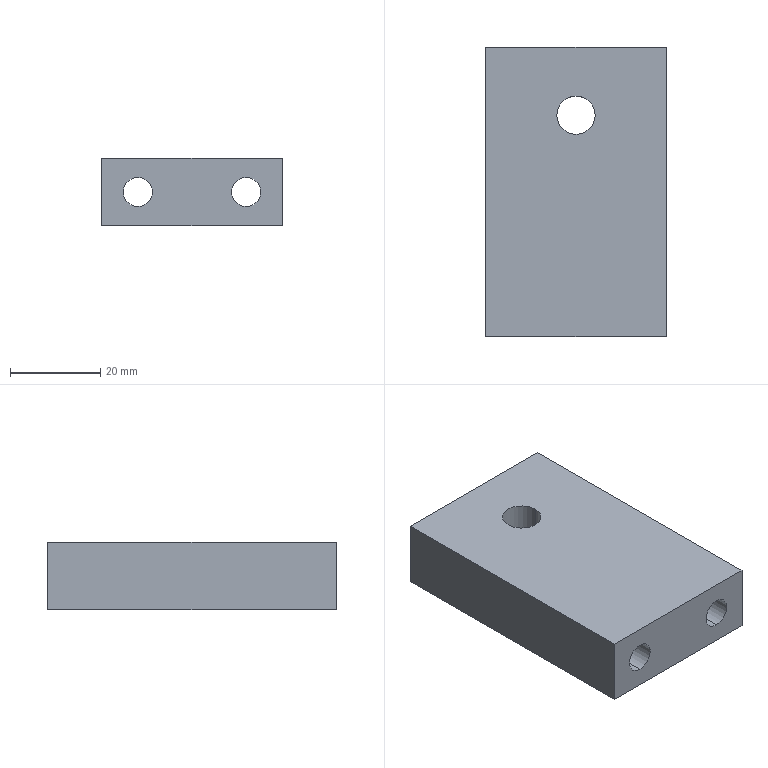Part | STEP file | 0245_205_Block | 1 solid | 12 faces | box 40 x 64 x 15 mm | volume 33301 mm3 | cylinder 6 | plane 6 | commonest cylinder face diameters 6.5 x4 8.5 x2
STEP:
#1=CARTESIAN_POINT('',(0.,0.,0.));
#2=DIRECTION('',(0.,0.,1.));
#3=DIRECTION('',(1.,0.,0.));
#4=AXIS2_PLACEMENT_3D('',#1,#2,#3);
#5=CARTESIAN_POINT('',(4.25,49.,-15.));
#6=VERTEX_POINT('',#5);
#7=CARTESIAN_POINT('',(4.25,49.,0.));
#8=VERTEX_POINT('',#7);
#9=CARTESIAN_POINT('',(4.25,49.,0.));
#10=DIRECTION('',(0.,0.,1.));
#11=VECTOR('',#10,1.);
#12=LINE('',#9,#11);
#13=CARTESIAN_POINT('',(0.,49.,0.));
#14=DIRECTION('',(0.,0.,1.));
#15=DIRECTION('',(1.,0.,0.));
#16=AXIS2_PLACEMENT_3D('',#13,#14,#15);
#17=CYLINDRICAL_SURFACE('',#16,4.25);
#18=CARTESIAN_POINT('',(6.283,0.));
#19=DIRECTION('',(0.,1.));
#20=VECTOR('',#19,1.);
#21=LINE('',#18,#20);
#22=(GEOMETRIC_REPRESENTATION_CONTEXT(2)PARAMETRIC_REPRESENTATION_CONTEXT()REPRESENTATION_CONTEXT('',''));
#23=DEFINITIONAL_REPRESENTATION('',(#21),#22);
#24=PCURVE('',#17,#23);
#25=CARTESIAN_POINT('',(0.,49.,0.));
#26=DIRECTION('',(0.,0.,1.));
#27=DIRECTION('',(1.,0.,0.));
#28=AXIS2_PLACEMENT_3D('',#25,#26,#27);
#29=CYLINDRICAL_SURFACE('',#28,4.25);
#30=CARTESIAN_POINT('',(0.,0.));
#31=DIRECTION('',(0.,1.));
#32=VECTOR('',#31,1.);
#33=LINE('',#30,#32);
#34=(GEOMETRIC_REPRESENTATION_CONTEXT(2)PARAMETRIC_REPRESENTATION_CONTEXT()REPRESENTATION_CONTEXT('',''));
#35=DEFINITIONAL_REPRESENTATION('',(#33),#34);
#36=PCURVE('',#29,#35);
#37=SURFACE_CURVE('',#12,(#24,#36),.PCURVE_S1.);
#38=EDGE_CURVE('',#6,#8,#37,.T.);
#39=ORIENTED_EDGE('',*,*,#38,.T.);
#40=CARTESIAN_POINT('',(-4.25,49.,0.));
#41=VERTEX_POINT('',#40);
#42=CARTESIAN_POINT('',(0.,49.,0.));
#43=DIRECTION('',(0.,0.,1.));
#44=DIRECTION('',(1.,0.,0.));
#45=AXIS2_PLACEMENT_3D('',#42,#43,#44);
#46=CIRCLE('',#45,4.25);
#47=CARTESIAN_POINT('',(0.,0.));
#48=DIRECTION('',(1.,0.));
#49=VECTOR('',#48,1.);
#50=LINE('',#47,#49);
#51=(GEOMETRIC_REPRESENTATION_CONTEXT(2)PARAMETRIC_REPRESENTATION_CONTEXT()REPRESENTATION_CONTEXT('',''));
#52=DEFINITIONAL_REPRESENTATION('',(#50),#51);
#53=PCURVE('',#17,#52);
#54=CARTESIAN_POINT('',(-20.,64.,0.));
#55=DIRECTION('',(0.,0.,-1.));
#56=DIRECTION('',(-1.,0.,0.));
#57=AXIS2_PLACEMENT_3D('',#54,#55,#56);
#58=PLANE('',#57);
#59=CARTESIAN_POINT('',(-24.25,-15.));
#60=CARTESIAN_POINT('',(-24.25,-7.639));
#61=CARTESIAN_POINT('',(-17.875,-11.319));
#62=CARTESIAN_POINT('',(-11.5,-15.));
#63=CARTESIAN_POINT('',(-17.875,-18.681));
#64=CARTESIAN_POINT('',(-24.25,-22.361));
#65=CARTESIAN_POINT('',(-24.25,-15.));
#66=(BOUNDED_CURVE()B_SPLINE_CURVE(2,(#59,#60,#61,#62,#63,#64,#65),.UNSPECIFIED.,.T.,.F.)B_SPLINE_CURVE_WITH_KNOTS((1,2,2,2,2,1),(-2.094,0.,2.094,4.189,6.283,8.378),.UNSPECIFIED.)CURVE()GEOMETRIC_REPRESENTATION_ITEM()RATIONAL_B_SPLINE_CURVE((1.,0.5,1.,0.5,1.,0.5,1.))REPRESENTATION_ITEM(''));
#67=(GEOMETRIC_REPRESENTATION_CONTEXT(2)PARAMETRIC_REPRESENTATION_CONTEXT()REPRESENTATION_CONTEXT('',''));
#68=DEFINITIONAL_REPRESENTATION('',(#66),#67);
#69=PCURVE('',#58,#68);
#70=SURFACE_CURVE('',#46,(#53,#69),.PCURVE_S1.);
#71=EDGE_CURVE('',#41,#8,#70,.T.);
#72=ORIENTED_EDGE('',*,*,#71,.F.);
#73=CARTESIAN_POINT('',(-4.25,49.,-15.));
#74=VERTEX_POINT('',#73);
#75=CARTESIAN_POINT('',(-4.25,49.,0.));
#76=DIRECTION('',(0.,0.,1.));
#77=VECTOR('',#76,1.);
#78=LINE('',#75,#77);
#79=CARTESIAN_POINT('',(3.142,0.));
#80=DIRECTION('',(0.,1.));
#81=VECTOR('',#80,1.);
#82=LINE('',#79,#81);
#83=(GEOMETRIC_REPRESENTATION_CONTEXT(2)PARAMETRIC_REPRESENTATION_CONTEXT()REPRESENTATION_CONTEXT('',''));
#84=DEFINITIONAL_REPRESENTATION('',(#82),#83);
#85=PCURVE('',#17,#84);
#86=CARTESIAN_POINT('',(3.142,0.));
#87=DIRECTION('',(0.,1.));
#88=VECTOR('',#87,1.);
#89=LINE('',#86,#88);
#90=(GEOMETRIC_REPRESENTATION_CONTEXT(2)PARAMETRIC_REPRESENTATION_CONTEXT()REPRESENTATION_CONTEXT('',''));
#91=DEFINITIONAL_REPRESENTATION('',(#89),#90);
#92=PCURVE('',#29,#91);
#93=SURFACE_CURVE('',#78,(#85,#92),.PCURVE_S1.);
#94=EDGE_CURVE('',#74,#41,#93,.T.);
#95=ORIENTED_EDGE('',*,*,#94,.F.);
#96=CARTESIAN_POINT('',(0.,49.,-15.));
#97=DIRECTION('',(0.,0.,1.));
#98=DIRECTION('',(1.,0.,0.));
#99=AXIS2_PLACEMENT_3D('',#96,#97,#98);
#100=CIRCLE('',#99,4.25);
#101=CARTESIAN_POINT('',(0.,-15.));
#102=DIRECTION('',(1.,0.));
#103=VECTOR('',#102,1.);
#104=LINE('',#101,#103);
#105=(GEOMETRIC_REPRESENTATION_CONTEXT(2)PARAMETRIC_REPRESENTATION_CONTEXT()REPRESENTATION_CONTEXT('',''));
#106=DEFINITIONAL_REPRESENTATION('',(#104),#105);
#107=PCURVE('',#17,#106);
#108=CARTESIAN_POINT('',(-20.,64.,-15.));
#109=DIRECTION('',(0.,0.,-1.));
#110=DIRECTION('',(-1.,0.,0.));
#111=AXIS2_PLACEMENT_3D('',#108,#109,#110);
#112=PLANE('',#111);
#113=CARTESIAN_POINT('',(-24.25,-15.));
#114=CARTESIAN_POINT('',(-24.25,-7.639));
#115=CARTESIAN_POINT('',(-17.875,-11.319));
#116=CARTESIAN_POINT('',(-11.5,-15.));
#117=CARTESIAN_POINT('',(-17.875,-18.681));
#118=CARTESIAN_POINT('',(-24.25,-22.361));
#119=CARTESIAN_POINT('',(-24.25,-15.));
#120=(BOUNDED_CURVE()B_SPLINE_CURVE(2,(#113,#114,#115,#116,#117,#118,#119),.UNSPECIFIED.,.T.,.F.)B_SPLINE_CURVE_WITH_KNOTS((1,2,2,2,2,1),(-2.094,0.,2.094,4.189,6.283,8.378),.UNSPECIFIED.)CURVE()GEOMETRIC_REPRESENTATION_ITEM()RATIONAL_B_SPLINE_CURVE((1.,0.5,1.,0.5,1.,0.5,1.))REPRESENTATION_ITEM(''));
#121=(GEOMETRIC_REPRESENTATION_CONTEXT(2)PARAMETRIC_REPRESENTATION_CONTEXT()REPRESENTATION_CONTEXT('',''));
#122=DEFINITIONAL_REPRESENTATION('',(#120),#121);
#123=PCURVE('',#112,#122);
#124=SURFACE_CURVE('',#100,(#107,#123),.PCURVE_S1.);
#125=EDGE_CURVE('',#74,#6,#124,.T.);
#126=ORIENTED_EDGE('',*,*,#125,.T.);
#127=EDGE_LOOP('',(#39,#72,#95,#126));
#128=FACE_BOUND('',#127,.F.);
#129=ADVANCED_FACE('',(#128),#17,.F.);
#130=CARTESIAN_POINT('',(-12.,0.,-4.25));
#131=VERTEX_POINT('',#130);
#132=CARTESIAN_POINT('',(-12.,64.,-4.25));
#133=VERTEX_POINT('',#132);
#134=CARTESIAN_POINT('',(-12.,64.,-4.25));
#135=DIRECTION('',(0.,1.,0.));
#136=VECTOR('',#135,1.);
#137=LINE('',#134,#136);
#138=CARTESIAN_POINT('',(-12.,64.,-7.5));
#139=DIRECTION('',(0.,1.,0.));
#140=DIRECTION('',(0.,0.,1.));
#141=AXIS2_PLACEMENT_3D('',#138,#139,#140);
#142=CYLINDRICAL_SURFACE('',#141,3.25);
#143=CARTESIAN_POINT('',(6.283,0.));
#144=DIRECTION('',(0.,1.));
#145=VECTOR('',#144,1.);
#146=LINE('',#143,#145);
#147=(GEOMETRIC_REPRESENTATION_CONTEXT(2)PARAMETRIC_REPRESENTATION_CONTEXT()REPRESENTATION_CONTEXT('',''));
#148=DEFINITIONAL_REPRESENTATION('',(#146),#147);
#149=PCURVE('',#142,#148);
#150=CARTESIAN_POINT('',(-12.,64.,-7.5));
#151=DIRECTION('',(0.,1.,0.));
#152=DIRECTION('',(0.,0.,1.));
#153=AXIS2_PLACEMENT_3D('',#150,#151,#152);
#154=CYLINDRICAL_SURFACE('',#153,3.25);
#155=CARTESIAN_POINT('',(0.,0.));
#156=DIRECTION('',(0.,1.));
#157=VECTOR('',#156,1.);
#158=LINE('',#155,#157);
#159=(GEOMETRIC_REPRESENTATION_CONTEXT(2)PARAMETRIC_REPRESENTATION_CONTEXT()REPRESENTATION_CONTEXT('',''));
#160=DEFINITIONAL_REPRESENTATION('',(#158),#159);
#161=PCURVE('',#154,#160);
#162=SURFACE_CURVE('',#137,(#149,#161),.PCURVE_S1.);
#163=EDGE_CURVE('',#131,#133,#162,.T.);
#164=ORIENTED_EDGE('',*,*,#163,.T.);
#165=CARTESIAN_POINT('',(-12.,64.,-10.75));
#166=VERTEX_POINT('',#165);
#167=CARTESIAN_POINT('',(-12.,64.,-7.5));
#168=DIRECTION('',(0.,1.,0.));
#169=DIRECTION('',(0.,0.,1.));
#170=AXIS2_PLACEMENT_3D('',#167,#168,#169);
#171=CIRCLE('',#170,3.25);
#172=CARTESIAN_POINT('',(0.,0.));
#173=DIRECTION('',(1.,0.));
#174=VECTOR('',#173,1.);
#175=LINE('',#172,#174);
#176=(GEOMETRIC_REPRESENTATION_CONTEXT(2)PARAMETRIC_REPRESENTATION_CONTEXT()REPRESENTATION_CONTEXT('',''));
#177=DEFINITIONAL_REPRESENTATION('',(#175),#176);
#178=PCURVE('',#142,#177);
#179=CARTESIAN_POINT('',(-20.,64.,-15.));
#180=DIRECTION('',(0.,1.,0.));
#181=DIRECTION('',(0.,0.,1.));
#182=AXIS2_PLACEMENT_3D('',#179,#180,#181);
#183=PLANE('',#182);
#184=CARTESIAN_POINT('',(7.5,8.));
#185=DIRECTION('',(1.,0.));
#186=AXIS2_PLACEMENT_2D('',#184,#185);
#187=CIRCLE('',#186,3.25);
#188=(GEOMETRIC_REPRESENTATION_CONTEXT(2)PARAMETRIC_REPRESENTATION_CONTEXT()REPRESENTATION_CONTEXT('',''));
#189=DEFINITIONAL_REPRESENTATION('',(#187),#188);
#190=PCURVE('',#183,#189);
#191=SURFACE_CURVE('',#171,(#178,#190),.PCURVE_S1.);
#192=EDGE_CURVE('',#166,#133,#191,.T.);
#193=ORIENTED_EDGE('',*,*,#192,.F.);
#194=CARTESIAN_POINT('',(-12.,0.,-10.75));
#195=VERTEX_POINT('',#194);
#196=CARTESIAN_POINT('',(-12.,64.,-10.75));
#197=DIRECTION('',(0.,1.,0.));
#198=VECTOR('',#197,1.);
#199=LINE('',#196,#198);
#200=CARTESIAN_POINT('',(3.142,0.));
#201=DIRECTION('',(0.,1.));
#202=VECTOR('',#201,1.);
#203=LINE('',#200,#202);
#204=(GEOMETRIC_REPRESENTATION_CONTEXT(2)PARAMETRIC_REPRESENTATION_CONTEXT()REPRESENTATION_CONTEXT('',''));
#205=DEFINITIONAL_REPRESENTATION('',(#203),#204);
#206=PCURVE('',#142,#205);
#207=CARTESIAN_POINT('',(3.142,0.));
#208=DIRECTION('',(0.,1.));
#209=VECTOR('',#208,1.);
#210=LINE('',#207,#209);
#211=(GEOMETRIC_REPRESENTATION_CONTEXT(2)PARAMETRIC_REPRESENTATION_CONTEXT()REPRESENTATION_CONTEXT('',''));
#212=DEFINITIONAL_REPRESENTATION('',(#210),#211);
#213=PCURVE('',#154,#212);
#214=SURFACE_CURVE('',#199,(#206,#213),.PCURVE_S1.);
#215=EDGE_CURVE('',#195,#166,#214,.T.);
#216=ORIENTED_EDGE('',*,*,#215,.F.);
#217=CARTESIAN_POINT('',(-12.,0.,-7.5));
#218=DIRECTION('',(0.,1.,0.));
#219=DIRECTION('',(0.,0.,1.));
#220=AXIS2_PLACEMENT_3D('',#217,#218,#219);
#221=CIRCLE('',#220,3.25);
#222=CARTESIAN_POINT('',(0.,-64.));
#223=DIRECTION('',(1.,0.));
#224=VECTOR('',#223,1.);
#225=LINE('',#222,#224);
#226=(GEOMETRIC_REPRESENTATION_CONTEXT(2)PARAMETRIC_REPRESENTATION_CONTEXT()REPRESENTATION_CONTEXT('',''));
#227=DEFINITIONAL_REPRESENTATION('',(#225),#226);
#228=PCURVE('',#142,#227);
#229=CARTESIAN_POINT('',(-20.,0.,-15.));
#230=DIRECTION('',(0.,-1.,0.));
#231=DIRECTION('',(0.,0.,-1.));
#232=AXIS2_PLACEMENT_3D('',#229,#230,#231);
#233=PLANE('',#232);
#234=CARTESIAN_POINT('',(-10.75,8.));
#235=CARTESIAN_POINT('',(-10.75,13.629));
#236=CARTESIAN_POINT('',(-5.875,10.815));
#237=CARTESIAN_POINT('',(-1.,8.));
#238=CARTESIAN_POINT('',(-5.875,5.185));
#239=CARTESIAN_POINT('',(-10.75,2.371));
#240=CARTESIAN_POINT('',(-10.75,8.));
#241=(BOUNDED_CURVE()B_SPLINE_CURVE(2,(#234,#235,#236,#237,#238,#239,#240),.UNSPECIFIED.,.T.,.F.)B_SPLINE_CURVE_WITH_KNOTS((1,2,2,2,2,1),(-2.094,0.,2.094,4.189,6.283,8.378),.UNSPECIFIED.)CURVE()GEOMETRIC_REPRESENTATION_ITEM()RATIONAL_B_SPLINE_CURVE((1.,0.5,1.,0.5,1.,0.5,1.))REPRESENTATION_ITEM(''));
#242=(GEOMETRIC_REPRESENTATION_CONTEXT(2)PARAMETRIC_REPRESENTATION_CONTEXT()REPRESENTATION_CONTEXT('',''));
#243=DEFINITIONAL_REPRESENTATION('',(#241),#242);
#244=PCURVE('',#233,#243);
#245=SURFACE_CURVE('',#221,(#228,#244),.PCURVE_S1.);
#246=EDGE_CURVE('',#195,#131,#245,.T.);
#247=ORIENTED_EDGE('',*,*,#246,.T.);
#248=EDGE_LOOP('',(#164,#193,#216,#247));
#249=FACE_BOUND('',#248,.F.);
#250=ADVANCED_FACE('',(#249),#142,.F.);
#251=CARTESIAN_POINT('',(12.,0.,-4.25));
#252=VERTEX_POINT('',#251);
#253=CARTESIAN_POINT('',(12.,64.,-4.25));
#254=VERTEX_POINT('',#253);
#255=CARTESIAN_POINT('',(12.,64.,-4.25));
#256=DIRECTION('',(0.,1.,0.));
#257=VECTOR('',#256,1.);
#258=LINE('',#255,#257);
#259=CARTESIAN_POINT('',(12.,64.,-7.5));
#260=DIRECTION('',(0.,1.,0.));
#261=DIRECTION('',(0.,0.,1.));
#262=AXIS2_PLACEMENT_3D('',#259,#260,#261);
#263=CYLINDRICAL_SURFACE('',#262,3.25);
#264=CARTESIAN_POINT('',(6.283,0.));
#265=DIRECTION('',(0.,1.));
#266=VECTOR('',#265,1.);
#267=LINE('',#264,#266);
#268=(GEOMETRIC_REPRESENTATION_CONTEXT(2)PARAMETRIC_REPRESENTATION_CONTEXT()REPRESENTATION_CONTEXT('',''));
#269=DEFINITIONAL_REPRESENTATION('',(#267),#268);
#270=PCURVE('',#263,#269);
#271=CARTESIAN_POINT('',(12.,64.,-7.5));
#272=DIRECTION('',(0.,1.,0.));
#273=DIRECTION('',(0.,0.,1.));
#274=AXIS2_PLACEMENT_3D('',#271,#272,#273);
#275=CYLINDRICAL_SURFACE('',#274,3.25);
#276=CARTESIAN_POINT('',(0.,0.));
#277=DIRECTION('',(0.,1.));
#278=VECTOR('',#277,1.);
#279=LINE('',#276,#278);
#280=(GEOMETRIC_REPRESENTATION_CONTEXT(2)PARAMETRIC_REPRESENTATION_CONTEXT()REPRESENTATION_CONTEXT('',''));
#281=DEFINITIONAL_REPRESENTATION('',(#279),#280);
#282=PCURVE('',#275,#281);
#283=SURFACE_CURVE('',#258,(#270,#282),.PCURVE_S1.);
#284=EDGE_CURVE('',#252,#254,#283,.T.);
#285=ORIENTED_EDGE('',*,*,#284,.T.);
#286=CARTESIAN_POINT('',(12.,64.,-10.75));
#287=VERTEX_POINT('',#286);
#288=CARTESIAN_POINT('',(12.,64.,-7.5));
#289=DIRECTION('',(0.,1.,0.));
#290=DIRECTION('',(0.,0.,1.));
#291=AXIS2_PLACEMENT_3D('',#288,#289,#290);
#292=CIRCLE('',#291,3.25);
#293=CARTESIAN_POINT('',(0.,0.));
#294=DIRECTION('',(1.,0.));
#295=VECTOR('',#294,1.);
#296=LINE('',#293,#295);
#297=(GEOMETRIC_REPRESENTATION_CONTEXT(2)PARAMETRIC_REPRESENTATION_CONTEXT()REPRESENTATION_CONTEXT('',''));
#298=DEFINITIONAL_REPRESENTATION('',(#296),#297);
#299=PCURVE('',#263,#298);
#300=CARTESIAN_POINT('',(7.5,32.));
#301=DIRECTION('',(1.,0.));
#302=AXIS2_PLACEMENT_2D('',#300,#301);
#303=CIRCLE('',#302,3.25);
#304=(GEOMETRIC_REPRESENTATION_CONTEXT(2)PARAMETRIC_REPRESENTATION_CONTEXT()REPRESENTATION_CONTEXT('',''));
#305=DEFINITIONAL_REPRESENTATION('',(#303),#304);
#306=PCURVE('',#183,#305);
#307=SURFACE_CURVE('',#292,(#299,#306),.PCURVE_S1.);
#308=EDGE_CURVE('',#287,#254,#307,.T.);
#309=ORIENTED_EDGE('',*,*,#308,.F.);
#310=CARTESIAN_POINT('',(12.,0.,-10.75));
#311=VERTEX_POINT('',#310);
#312=CARTESIAN_POINT('',(12.,64.,-10.75));
#313=DIRECTION('',(0.,1.,0.));
#314=VECTOR('',#313,1.);
#315=LINE('',#312,#314);
#316=CARTESIAN_POINT('',(3.142,0.));
#317=DIRECTION('',(0.,1.));
#318=VECTOR('',#317,1.);
#319=LINE('',#316,#318);
#320=(GEOMETRIC_REPRESENTATION_CONTEXT(2)PARAMETRIC_REPRESENTATION_CONTEXT()REPRESENTATION_CONTEXT('',''));
#321=DEFINITIONAL_REPRESENTATION('',(#319),#320);
#322=PCURVE('',#263,#321);
#323=CARTESIAN_POINT('',(3.142,0.));
#324=DIRECTION('',(0.,1.));
#325=VECTOR('',#324,1.);
#326=LINE('',#323,#325);
#327=(GEOMETRIC_REPRESENTATION_CONTEXT(2)PARAMETRIC_REPRESENTATION_CONTEXT()REPRESENTATION_CONTEXT('',''));
#328=DEFINITIONAL_REPRESENTATION('',(#326),#327);
#329=PCURVE('',#275,#328);
#330=SURFACE_CURVE('',#315,(#322,#329),.PCURVE_S1.);
#331=EDGE_CURVE('',#311,#287,#330,.T.);
#332=ORIENTED_EDGE('',*,*,#331,.F.);
#333=CARTESIAN_POINT('',(12.,0.,-7.5));
#334=DIRECTION('',(0.,1.,0.));
#335=DIRECTION('',(0.,0.,1.));
#336=AXIS2_PLACEMENT_3D('',#333,#334,#335);
#337=CIRCLE('',#336,3.25);
#338=CARTESIAN_POINT('',(0.,-64.));
#339=DIRECTION('',(1.,0.));
#340=VECTOR('',#339,1.);
#341=LINE('',#338,#340);
#342=(GEOMETRIC_REPRESENTATION_CONTEXT(2)PARAMETRIC_REPRESENTATION_CONTEXT()REPRESENTATION_CONTEXT('',''));
#343=DEFINITIONAL_REPRESENTATION('',(#341),#342);
#344=PCURVE('',#263,#343);
#345=CARTESIAN_POINT('',(-10.75,32.));
#346=CARTESIAN_POINT('',(-10.75,37.629));
#347=CARTESIAN_POINT('',(-5.875,34.815));
#348=CARTESIAN_POINT('',(-1.,32.));
#349=CARTESIAN_POINT('',(-5.875,29.185));
#350=CARTESIAN_POINT('',(-10.75,26.371));
#351=CARTESIAN_POINT('',(-10.75,32.));
#352=(BOUNDED_CURVE()B_SPLINE_CURVE(2,(#345,#346,#347,#348,#349,#350,#351),.UNSPECIFIED.,.T.,.F.)B_SPLINE_CURVE_WITH_KNOTS((1,2,2,2,2,1),(-2.094,0.,2.094,4.189,6.283,8.378),.UNSPECIFIED.)CURVE()GEOMETRIC_REPRESENTATION_ITEM()RATIONAL_B_SPLINE_CURVE((1.,0.5,1.,0.5,1.,0.5,1.))REPRESENTATION_ITEM(''));
#353=(GEOMETRIC_REPRESENTATION_CONTEXT(2)PARAMETRIC_REPRESENTATION_CONTEXT()REPRESENTATION_CONTEXT('',''));
#354=DEFINITIONAL_REPRESENTATION('',(#352),#353);
#355=PCURVE('',#233,#354);
#356=SURFACE_CURVE('',#337,(#344,#355),.PCURVE_S1.);
#357=EDGE_CURVE('',#311,#252,#356,.T.);
#358=ORIENTED_EDGE('',*,*,#357,.T.);
#359=EDGE_LOOP('',(#285,#309,#332,#358));
#360=FACE_BOUND('',#359,.F.);
#361=ADVANCED_FACE('',(#360),#263,.F.);
#362=CARTESIAN_POINT('',(-20.,64.,0.));
#363=VERTEX_POINT('',#362);
#364=CARTESIAN_POINT('',(-20.,0.,0.));
#365=VERTEX_POINT('',#364);
#366=CARTESIAN_POINT('',(-20.,0.,0.));
#367=DIRECTION('',(0.,-1.,0.));
#368=VECTOR('',#367,1.);
#369=LINE('',#366,#368);
#370=CARTESIAN_POINT('',(-20.,0.,-15.));
#371=DIRECTION('',(-1.,0.,0.));
#372=DIRECTION('',(0.,0.,1.));
#373=AXIS2_PLACEMENT_3D('',#370,#371,#372);
#374=PLANE('',#373);
#375=CARTESIAN_POINT('',(15.,0.));
#376=DIRECTION('',(0.,-1.));
#377=VECTOR('',#376,1.);
#378=LINE('',#375,#377);
#379=(GEOMETRIC_REPRESENTATION_CONTEXT(2)PARAMETRIC_REPRESENTATION_CONTEXT()REPRESENTATION_CONTEXT('',''));
#380=DEFINITIONAL_REPRESENTATION('',(#378),#379);
#381=PCURVE('',#374,#380);
#382=CARTESIAN_POINT('',(0.,-64.));
#383=DIRECTION('',(0.,-1.));
#384=VECTOR('',#383,1.);
#385=LINE('',#382,#384);
#386=(GEOMETRIC_REPRESENTATION_CONTEXT(2)PARAMETRIC_REPRESENTATION_CONTEXT()REPRESENTATION_CONTEXT('',''));
#387=DEFINITIONAL_REPRESENTATION('',(#385),#386);
#388=PCURVE('',#58,#387);
#389=SURFACE_CURVE('',#369,(#381,#388),.PCURVE_S1.);
#390=EDGE_CURVE('',#363,#365,#389,.T.);
#391=ORIENTED_EDGE('',*,*,#390,.F.);
#392=CARTESIAN_POINT('',(-20.,64.,-15.));
#393=VERTEX_POINT('',#392);
#394=CARTESIAN_POINT('',(-20.,64.,-15.));
#395=DIRECTION('',(0.,0.,1.));
#396=VECTOR('',#395,1.);
#397=LINE('',#394,#396);
#398=CARTESIAN_POINT('',(0.,64.));
#399=DIRECTION('',(1.,0.));
#400=VECTOR('',#399,1.);
#401=LINE('',#398,#400);
#402=(GEOMETRIC_REPRESENTATION_CONTEXT(2)PARAMETRIC_REPRESENTATION_CONTEXT()REPRESENTATION_CONTEXT('',''));
#403=DEFINITIONAL_REPRESENTATION('',(#401),#402);
#404=PCURVE('',#374,#403);
#405=CARTESIAN_POINT('',(0.,0.));
#406=DIRECTION('',(1.,0.));
#407=VECTOR('',#406,1.);
#408=LINE('',#405,#407);
#409=(GEOMETRIC_REPRESENTATION_CONTEXT(2)PARAMETRIC_REPRESENTATION_CONTEXT()REPRESENTATION_CONTEXT('',''));
#410=DEFINITIONAL_REPRESENTATION('',(#408),#409);
#411=PCURVE('',#183,#410);
#412=SURFACE_CURVE('',#397,(#404,#411),.PCURVE_S1.);
#413=EDGE_CURVE('',#393,#363,#412,.T.);
#414=ORIENTED_EDGE('',*,*,#413,.F.);
#415=CARTESIAN_POINT('',(-20.,0.,-15.));
#416=VERTEX_POINT('',#415);
#417=CARTESIAN_POINT('',(-20.,0.,-15.));
#418=DIRECTION('',(0.,-1.,0.));
#419=VECTOR('',#418,1.);
#420=LINE('',#417,#419);
#421=CARTESIAN_POINT('',(0.,0.));
#422=DIRECTION('',(0.,-1.));
#423=VECTOR('',#422,1.);
#424=LINE('',#421,#423);
#425=(GEOMETRIC_REPRESENTATION_CONTEXT(2)PARAMETRIC_REPRESENTATION_CONTEXT()REPRESENTATION_CONTEXT('',''));
#426=DEFINITIONAL_REPRESENTATION('',(#424),#425);
#427=PCURVE('',#374,#426);
#428=CARTESIAN_POINT('',(0.,-64.));
#429=DIRECTION('',(0.,-1.));
#430=VECTOR('',#429,1.);
#431=LINE('',#428,#430);
#432=(GEOMETRIC_REPRESENTATION_CONTEXT(2)PARAMETRIC_REPRESENTATION_CONTEXT()REPRESENTATION_CONTEXT('',''));
#433=DEFINITIONAL_REPRESENTATION('',(#431),#432);
#434=PCURVE('',#112,#433);
#435=SURFACE_CURVE('',#420,(#427,#434),.PCURVE_S1.);
#436=EDGE_CURVE('',#393,#416,#435,.T.);
#437=ORIENTED_EDGE('',*,*,#436,.T.);
#438=CARTESIAN_POINT('',(-20.,0.,-15.));
#439=DIRECTION('',(0.,0.,1.));
#440=VECTOR('',#439,1.);
#441=LINE('',#438,#440);
#442=CARTESIAN_POINT('',(0.,0.));
#443=DIRECTION('',(1.,0.));
#444=VECTOR('',#443,1.);
#445=LINE('',#442,#444);
#446=(GEOMETRIC_REPRESENTATION_CONTEXT(2)PARAMETRIC_REPRESENTATION_CONTEXT()REPRESENTATION_CONTEXT('',''));
#447=DEFINITIONAL_REPRESENTATION('',(#445),#446);
#448=PCURVE('',#374,#447);
#449=CARTESIAN_POINT('',(0.,0.));
#450=DIRECTION('',(-1.,0.));
#451=VECTOR('',#450,1.);
#452=LINE('',#449,#451);
#453=(GEOMETRIC_REPRESENTATION_CONTEXT(2)PARAMETRIC_REPRESENTATION_CONTEXT()REPRESENTATION_CONTEXT('',''));
#454=DEFINITIONAL_REPRESENTATION('',(#452),#453);
#455=PCURVE('',#233,#454);
#456=SURFACE_CURVE('',#441,(#448,#455),.PCURVE_S1.);
#457=EDGE_CURVE('',#416,#365,#456,.T.);
#458=ORIENTED_EDGE('',*,*,#457,.T.);
#459=EDGE_LOOP('',(#391,#414,#437,#458));
#460=FACE_BOUND('',#459,.T.);
#461=ADVANCED_FACE('',(#460),#374,.T.);
#462=CARTESIAN_POINT('',(-12.,64.,-7.5));
#463=DIRECTION('',(0.,1.,0.));
#464=DIRECTION('',(0.,0.,1.));
#465=AXIS2_PLACEMENT_3D('',#462,#463,#464);
#466=CIRCLE('',#465,3.25);
#467=CARTESIAN_POINT('',(7.5,8.));
#468=DIRECTION('',(1.,0.));
#469=AXIS2_PLACEMENT_2D('',#467,#468);
#470=CIRCLE('',#469,3.25);
#471=(GEOMETRIC_REPRESENTATION_CONTEXT(2)PARAMETRIC_REPRESENTATION_CONTEXT()REPRESENTATION_CONTEXT('',''));
#472=DEFINITIONAL_REPRESENTATION('',(#470),#471);
#473=PCURVE('',#183,#472);
#474=CARTESIAN_POINT('',(0.,0.));
#475=DIRECTION('',(1.,0.));
#476=VECTOR('',#475,1.);
#477=LINE('',#474,#476);
#478=(GEOMETRIC_REPRESENTATION_CONTEXT(2)PARAMETRIC_REPRESENTATION_CONTEXT()REPRESENTATION_CONTEXT('',''));
#479=DEFINITIONAL_REPRESENTATION('',(#477),#478);
#480=PCURVE('',#154,#479);
#481=SURFACE_CURVE('',#466,(#473,#480),.PCURVE_S1.);
#482=EDGE_CURVE('',#133,#166,#481,.T.);
#483=ORIENTED_EDGE('',*,*,#482,.F.);
#484=ORIENTED_EDGE('',*,*,#192,.F.);
#485=EDGE_LOOP('',(#483,#484));
#486=FACE_BOUND('',#485,.T.);
#487=CARTESIAN_POINT('',(12.,64.,-7.5));
#488=DIRECTION('',(0.,1.,0.));
#489=DIRECTION('',(0.,0.,1.));
#490=AXIS2_PLACEMENT_3D('',#487,#488,#489);
#491=CIRCLE('',#490,3.25);
#492=CARTESIAN_POINT('',(7.5,32.));
#493=DIRECTION('',(1.,0.));
#494=AXIS2_PLACEMENT_2D('',#492,#493);
#495=CIRCLE('',#494,3.25);
#496=(GEOMETRIC_REPRESENTATION_CONTEXT(2)PARAMETRIC_REPRESENTATION_CONTEXT()REPRESENTATION_CONTEXT('',''));
#497=DEFINITIONAL_REPRESENTATION('',(#495),#496);
#498=PCURVE('',#183,#497);
#499=CARTESIAN_POINT('',(0.,0.));
#500=DIRECTION('',(1.,0.));
#501=VECTOR('',#500,1.);
#502=LINE('',#499,#501);
#503=(GEOMETRIC_REPRESENTATION_CONTEXT(2)PARAMETRIC_REPRESENTATION_CONTEXT()REPRESENTATION_CONTEXT('',''));
#504=DEFINITIONAL_REPRESENTATION('',(#502),#503);
#505=PCURVE('',#275,#504);
#506=SURFACE_CURVE('',#491,(#498,#505),.PCURVE_S1.);
#507=EDGE_CURVE('',#254,#287,#506,.T.);
#508=ORIENTED_EDGE('',*,*,#507,.F.);
#509=ORIENTED_EDGE('',*,*,#308,.F.);
#510=EDGE_LOOP('',(#508,#509));
#511=FACE_BOUND('',#510,.T.);
#512=CARTESIAN_POINT('',(20.,64.,0.));
#513=VERTEX_POINT('',#512);
#514=CARTESIAN_POINT('',(-20.,64.,0.));
#515=DIRECTION('',(-1.,0.,0.));
#516=VECTOR('',#515,1.);
#517=LINE('',#514,#516);
#518=CARTESIAN_POINT('',(15.,0.));
#519=DIRECTION('',(0.,-1.));
#520=VECTOR('',#519,1.);
#521=LINE('',#518,#520);
#522=(GEOMETRIC_REPRESENTATION_CONTEXT(2)PARAMETRIC_REPRESENTATION_CONTEXT()REPRESENTATION_CONTEXT('',''));
#523=DEFINITIONAL_REPRESENTATION('',(#521),#522);
#524=PCURVE('',#183,#523);
#525=CARTESIAN_POINT('',(0.,0.));
#526=DIRECTION('',(1.,0.));
#527=VECTOR('',#526,1.);
#528=LINE('',#525,#527);
#529=(GEOMETRIC_REPRESENTATION_CONTEXT(2)PARAMETRIC_REPRESENTATION_CONTEXT()REPRESENTATION_CONTEXT('',''));
#530=DEFINITIONAL_REPRESENTATION('',(#528),#529);
#531=PCURVE('',#58,#530);
#532=SURFACE_CURVE('',#517,(#524,#531),.PCURVE_S1.);
#533=EDGE_CURVE('',#513,#363,#532,.T.);
#534=ORIENTED_EDGE('',*,*,#533,.F.);
#535=CARTESIAN_POINT('',(20.,64.,-15.));
#536=VERTEX_POINT('',#535);
#537=CARTESIAN_POINT('',(20.,64.,-15.));
#538=DIRECTION('',(0.,0.,1.));
#539=VECTOR('',#538,1.);
#540=LINE('',#537,#539);
#541=CARTESIAN_POINT('',(0.,40.));
#542=DIRECTION('',(1.,0.));
#543=VECTOR('',#542,1.);
#544=LINE('',#541,#543);
#545=(GEOMETRIC_REPRESENTATION_CONTEXT(2)PARAMETRIC_REPRESENTATION_CONTEXT()REPRESENTATION_CONTEXT('',''));
#546=DEFINITIONAL_REPRESENTATION('',(#544),#545);
#547=PCURVE('',#183,#546);
#548=CARTESIAN_POINT('',(20.,0.,-15.));
#549=DIRECTION('',(1.,0.,0.));
#550=DIRECTION('',(0.,0.,-1.));
#551=AXIS2_PLACEMENT_3D('',#548,#549,#550);
#552=PLANE('',#551);
#553=CARTESIAN_POINT('',(0.,64.));
#554=DIRECTION('',(-1.,0.));
#555=VECTOR('',#554,1.);
#556=LINE('',#553,#555);
#557=(GEOMETRIC_REPRESENTATION_CONTEXT(2)PARAMETRIC_REPRESENTATION_CONTEXT()REPRESENTATION_CONTEXT('',''));
#558=DEFINITIONAL_REPRESENTATION('',(#556),#557);
#559=PCURVE('',#552,#558);
#560=SURFACE_CURVE('',#540,(#547,#559),.PCURVE_S1.);
#561=EDGE_CURVE('',#536,#513,#560,.T.);
#562=ORIENTED_EDGE('',*,*,#561,.F.);
#563=CARTESIAN_POINT('',(-20.,64.,-15.));
#564=DIRECTION('',(-1.,0.,0.));
#565=VECTOR('',#564,1.);
#566=LINE('',#563,#565);
#567=CARTESIAN_POINT('',(0.,0.));
#568=DIRECTION('',(0.,-1.));
#569=VECTOR('',#568,1.);
#570=LINE('',#567,#569);
#571=(GEOMETRIC_REPRESENTATION_CONTEXT(2)PARAMETRIC_REPRESENTATION_CONTEXT()REPRESENTATION_CONTEXT('',''));
#572=DEFINITIONAL_REPRESENTATION('',(#570),#571);
#573=PCURVE('',#183,#572);
#574=CARTESIAN_POINT('',(0.,0.));
#575=DIRECTION('',(1.,0.));
#576=VECTOR('',#575,1.);
#577=LINE('',#574,#576);
#578=(GEOMETRIC_REPRESENTATION_CONTEXT(2)PARAMETRIC_REPRESENTATION_CONTEXT()REPRESENTATION_CONTEXT('',''));
#579=DEFINITIONAL_REPRESENTATION('',(#577),#578);
#580=PCURVE('',#112,#579);
#581=SURFACE_CURVE('',#566,(#573,#580),.PCURVE_S1.);
#582=EDGE_CURVE('',#536,#393,#581,.T.);
#583=ORIENTED_EDGE('',*,*,#582,.T.);
#584=ORIENTED_EDGE('',*,*,#413,.T.);
#585=EDGE_LOOP('',(#534,#562,#583,#584));
#586=FACE_BOUND('',#585,.T.);
#587=ADVANCED_FACE('',(#486,#511,#586),#183,.T.);
#588=CARTESIAN_POINT('',(20.,0.,0.));
#589=VERTEX_POINT('',#588);
#590=CARTESIAN_POINT('',(20.,0.,0.));
#591=DIRECTION('',(0.,1.,0.));
#592=VECTOR('',#591,1.);
#593=LINE('',#590,#592);
#594=CARTESIAN_POINT('',(-15.,0.));
#595=DIRECTION('',(0.,1.));
#596=VECTOR('',#595,1.);
#597=LINE('',#594,#596);
#598=(GEOMETRIC_REPRESENTATION_CONTEXT(2)PARAMETRIC_REPRESENTATION_CONTEXT()REPRESENTATION_CONTEXT('',''));
#599=DEFINITIONAL_REPRESENTATION('',(#597),#598);
#600=PCURVE('',#552,#599);
#601=CARTESIAN_POINT('',(-40.,-64.));
#602=DIRECTION('',(0.,1.));
#603=VECTOR('',#602,1.);
#604=LINE('',#601,#603);
#605=(GEOMETRIC_REPRESENTATION_CONTEXT(2)PARAMETRIC_REPRESENTATION_CONTEXT()REPRESENTATION_CONTEXT('',''));
#606=DEFINITIONAL_REPRESENTATION('',(#604),#605);
#607=PCURVE('',#58,#606);
#608=SURFACE_CURVE('',#593,(#600,#607),.PCURVE_S1.);
#609=EDGE_CURVE('',#589,#513,#608,.T.);
#610=ORIENTED_EDGE('',*,*,#609,.F.);
#611=CARTESIAN_POINT('',(20.,0.,-15.));
#612=VERTEX_POINT('',#611);
#613=CARTESIAN_POINT('',(20.,0.,-15.));
#614=DIRECTION('',(0.,0.,1.));
#615=VECTOR('',#614,1.);
#616=LINE('',#613,#615);
#617=CARTESIAN_POINT('',(0.,0.));
#618=DIRECTION('',(-1.,0.));
#619=VECTOR('',#618,1.);
#620=LINE('',#617,#619);
#621=(GEOMETRIC_REPRESENTATION_CONTEXT(2)PARAMETRIC_REPRESENTATION_CONTEXT()REPRESENTATION_CONTEXT('',''));
#622=DEFINITIONAL_REPRESENTATION('',(#620),#621);
#623=PCURVE('',#552,#622);
#624=CARTESIAN_POINT('',(0.,40.));
#625=DIRECTION('',(-1.,0.));
#626=VECTOR('',#625,1.);
#627=LINE('',#624,#626);
#628=(GEOMETRIC_REPRESENTATION_CONTEXT(2)PARAMETRIC_REPRESENTATION_CONTEXT()REPRESENTATION_CONTEXT('',''));
#629=DEFINITIONAL_REPRESENTATION('',(#627),#628);
#630=PCURVE('',#233,#629);
#631=SURFACE_CURVE('',#616,(#623,#630),.PCURVE_S1.);
#632=EDGE_CURVE('',#612,#589,#631,.T.);
#633=ORIENTED_EDGE('',*,*,#632,.F.);
#634=CARTESIAN_POINT('',(20.,0.,-15.));
#635=DIRECTION('',(0.,1.,0.));
#636=VECTOR('',#635,1.);
#637=LINE('',#634,#636);
#638=CARTESIAN_POINT('',(0.,0.));
#639=DIRECTION('',(0.,1.));
#640=VECTOR('',#639,1.);
#641=LINE('',#638,#640);
#642=(GEOMETRIC_REPRESENTATION_CONTEXT(2)PARAMETRIC_REPRESENTATION_CONTEXT()REPRESENTATION_CONTEXT('',''));
#643=DEFINITIONAL_REPRESENTATION('',(#641),#642);
#644=PCURVE('',#552,#643);
#645=CARTESIAN_POINT('',(-40.,-64.));
#646=DIRECTION('',(0.,1.));
#647=VECTOR('',#646,1.);
#648=LINE('',#645,#647);
#649=(GEOMETRIC_REPRESENTATION_CONTEXT(2)PARAMETRIC_REPRESENTATION_CONTEXT()REPRESENTATION_CONTEXT('',''));
#650=DEFINITIONAL_REPRESENTATION('',(#648),#649);
#651=PCURVE('',#112,#650);
#652=SURFACE_CURVE('',#637,(#644,#651),.PCURVE_S1.);
#653=EDGE_CURVE('',#612,#536,#652,.T.);
#654=ORIENTED_EDGE('',*,*,#653,.T.);
#655=ORIENTED_EDGE('',*,*,#561,.T.);
#656=EDGE_LOOP('',(#610,#633,#654,#655));
#657=FACE_BOUND('',#656,.T.);
#658=ADVANCED_FACE('',(#657),#552,.T.);
#659=CARTESIAN_POINT('',(-12.,0.,-7.5));
#660=DIRECTION('',(0.,1.,0.));
#661=DIRECTION('',(0.,0.,1.));
#662=AXIS2_PLACEMENT_3D('',#659,#660,#661);
#663=CIRCLE('',#662,3.25);
#664=CARTESIAN_POINT('',(-10.75,8.));
#665=CARTESIAN_POINT('',(-10.75,13.629));
#666=CARTESIAN_POINT('',(-5.875,10.815));
#667=CARTESIAN_POINT('',(-1.,8.));
#668=CARTESIAN_POINT('',(-5.875,5.185));
#669=CARTESIAN_POINT('',(-10.75,2.371));
#670=CARTESIAN_POINT('',(-10.75,8.));
#671=(BOUNDED_CURVE()B_SPLINE_CURVE(2,(#664,#665,#666,#667,#668,#669,#670),.UNSPECIFIED.,.T.,.F.)B_SPLINE_CURVE_WITH_KNOTS((1,2,2,2,2,1),(-2.094,0.,2.094,4.189,6.283,8.378),.UNSPECIFIED.)CURVE()GEOMETRIC_REPRESENTATION_ITEM()RATIONAL_B_SPLINE_CURVE((1.,0.5,1.,0.5,1.,0.5,1.))REPRESENTATION_ITEM(''));
#672=(GEOMETRIC_REPRESENTATION_CONTEXT(2)PARAMETRIC_REPRESENTATION_CONTEXT()REPRESENTATION_CONTEXT('',''));
#673=DEFINITIONAL_REPRESENTATION('',(#671),#672);
#674=PCURVE('',#233,#673);
#675=CARTESIAN_POINT('',(0.,-64.));
#676=DIRECTION('',(1.,0.));
#677=VECTOR('',#676,1.);
#678=LINE('',#675,#677);
#679=(GEOMETRIC_REPRESENTATION_CONTEXT(2)PARAMETRIC_REPRESENTATION_CONTEXT()REPRESENTATION_CONTEXT('',''));
#680=DEFINITIONAL_REPRESENTATION('',(#678),#679);
#681=PCURVE('',#154,#680);
#682=SURFACE_CURVE('',#663,(#674,#681),.PCURVE_S1.);
#683=EDGE_CURVE('',#131,#195,#682,.T.);
#684=ORIENTED_EDGE('',*,*,#683,.T.);
#685=ORIENTED_EDGE('',*,*,#246,.T.);
#686=EDGE_LOOP('',(#684,#685));
#687=FACE_BOUND('',#686,.T.);
#688=CARTESIAN_POINT('',(12.,0.,-7.5));
#689=DIRECTION('',(0.,1.,0.));
#690=DIRECTION('',(0.,0.,1.));
#691=AXIS2_PLACEMENT_3D('',#688,#689,#690);
#692=CIRCLE('',#691,3.25);
#693=CARTESIAN_POINT('',(-10.75,32.));
#694=CARTESIAN_POINT('',(-10.75,37.629));
#695=CARTESIAN_POINT('',(-5.875,34.815));
#696=CARTESIAN_POINT('',(-1.,32.));
#697=CARTESIAN_POINT('',(-5.875,29.185));
#698=CARTESIAN_POINT('',(-10.75,26.371));
#699=CARTESIAN_POINT('',(-10.75,32.));
#700=(BOUNDED_CURVE()B_SPLINE_CURVE(2,(#693,#694,#695,#696,#697,#698,#699),.UNSPECIFIED.,.T.,.F.)B_SPLINE_CURVE_WITH_KNOTS((1,2,2,2,2,1),(-2.094,0.,2.094,4.189,6.283,8.378),.UNSPECIFIED.)CURVE()GEOMETRIC_REPRESENTATION_ITEM()RATIONAL_B_SPLINE_CURVE((1.,0.5,1.,0.5,1.,0.5,1.))REPRESENTATION_ITEM(''));
#701=(GEOMETRIC_REPRESENTATION_CONTEXT(2)PARAMETRIC_REPRESENTATION_CONTEXT()REPRESENTATION_CONTEXT('',''));
#702=DEFINITIONAL_REPRESENTATION('',(#700),#701);
#703=PCURVE('',#233,#702);
#704=CARTESIAN_POINT('',(0.,-64.));
#705=DIRECTION('',(1.,0.));
#706=VECTOR('',#705,1.);
#707=LINE('',#704,#706);
#708=(GEOMETRIC_REPRESENTATION_CONTEXT(2)PARAMETRIC_REPRESENTATION_CONTEXT()REPRESENTATION_CONTEXT('',''));
#709=DEFINITIONAL_REPRESENTATION('',(#707),#708);
#710=PCURVE('',#275,#709);
#711=SURFACE_CURVE('',#692,(#703,#710),.PCURVE_S1.);
#712=EDGE_CURVE('',#252,#311,#711,.T.);
#713=ORIENTED_EDGE('',*,*,#712,.T.);
#714=ORIENTED_EDGE('',*,*,#357,.T.);
#715=EDGE_LOOP('',(#713,#714));
#716=FACE_BOUND('',#715,.T.);
#717=CARTESIAN_POINT('',(-20.,0.,0.));
#718=DIRECTION('',(1.,0.,0.));
#719=VECTOR('',#718,1.);
#720=LINE('',#717,#719);
#721=CARTESIAN_POINT('',(-15.,0.));
#722=DIRECTION('',(0.,1.));
#723=VECTOR('',#722,1.);
#724=LINE('',#721,#723);
#725=(GEOMETRIC_REPRESENTATION_CONTEXT(2)PARAMETRIC_REPRESENTATION_CONTEXT()REPRESENTATION_CONTEXT('',''));
#726=DEFINITIONAL_REPRESENTATION('',(#724),#725);
#727=PCURVE('',#233,#726);
#728=CARTESIAN_POINT('',(0.,-64.));
#729=DIRECTION('',(-1.,0.));
#730=VECTOR('',#729,1.);
#731=LINE('',#728,#730);
#732=(GEOMETRIC_REPRESENTATION_CONTEXT(2)PARAMETRIC_REPRESENTATION_CONTEXT()REPRESENTATION_CONTEXT('',''));
#733=DEFINITIONAL_REPRESENTATION('',(#731),#732);
#734=PCURVE('',#58,#733);
#735=SURFACE_CURVE('',#720,(#727,#734),.PCURVE_S1.);
#736=EDGE_CURVE('',#365,#589,#735,.T.);
#737=ORIENTED_EDGE('',*,*,#736,.F.);
#738=ORIENTED_EDGE('',*,*,#457,.F.);
#739=CARTESIAN_POINT('',(-20.,0.,-15.));
#740=DIRECTION('',(1.,0.,0.));
#741=VECTOR('',#740,1.);
#742=LINE('',#739,#741);
#743=CARTESIAN_POINT('',(0.,0.));
#744=DIRECTION('',(0.,1.));
#745=VECTOR('',#744,1.);
#746=LINE('',#743,#745);
#747=(GEOMETRIC_REPRESENTATION_CONTEXT(2)PARAMETRIC_REPRESENTATION_CONTEXT()REPRESENTATION_CONTEXT('',''));
#748=DEFINITIONAL_REPRESENTATION('',(#746),#747);
#749=PCURVE('',#233,#748);
#750=CARTESIAN_POINT('',(0.,-64.));
#751=DIRECTION('',(-1.,0.));
#752=VECTOR('',#751,1.);
#753=LINE('',#750,#752);
#754=(GEOMETRIC_REPRESENTATION_CONTEXT(2)PARAMETRIC_REPRESENTATION_CONTEXT()REPRESENTATION_CONTEXT('',''));
#755=DEFINITIONAL_REPRESENTATION('',(#753),#754);
#756=PCURVE('',#112,#755);
#757=SURFACE_CURVE('',#742,(#749,#756),.PCURVE_S1.);
#758=EDGE_CURVE('',#416,#612,#757,.T.);
#759=ORIENTED_EDGE('',*,*,#758,.T.);
#760=ORIENTED_EDGE('',*,*,#632,.T.);
#761=EDGE_LOOP('',(#737,#738,#759,#760));
#762=FACE_BOUND('',#761,.T.);
#763=ADVANCED_FACE('',(#687,#716,#762),#233,.T.);
#764=CARTESIAN_POINT('',(0.,49.,-15.));
#765=DIRECTION('',(0.,0.,1.));
#766=DIRECTION('',(1.,0.,0.));
#767=AXIS2_PLACEMENT_3D('',#764,#765,#766);
#768=CIRCLE('',#767,4.25);
#769=CARTESIAN_POINT('',(-24.25,-15.));
#770=CARTESIAN_POINT('',(-24.25,-7.639));
#771=CARTESIAN_POINT('',(-17.875,-11.319));
#772=CARTESIAN_POINT('',(-11.5,-15.));
#773=CARTESIAN_POINT('',(-17.875,-18.681));
#774=CARTESIAN_POINT('',(-24.25,-22.361));
#775=CARTESIAN_POINT('',(-24.25,-15.));
#776=(BOUNDED_CURVE()B_SPLINE_CURVE(2,(#769,#770,#771,#772,#773,#774,#775),.UNSPECIFIED.,.T.,.F.)B_SPLINE_CURVE_WITH_KNOTS((1,2,2,2,2,1),(-2.094,0.,2.094,4.189,6.283,8.378),.UNSPECIFIED.)CURVE()GEOMETRIC_REPRESENTATION_ITEM()RATIONAL_B_SPLINE_CURVE((1.,0.5,1.,0.5,1.,0.5,1.))REPRESENTATION_ITEM(''));
#777=(GEOMETRIC_REPRESENTATION_CONTEXT(2)PARAMETRIC_REPRESENTATION_CONTEXT()REPRESENTATION_CONTEXT('',''));
#778=DEFINITIONAL_REPRESENTATION('',(#776),#777);
#779=PCURVE('',#112,#778);
#780=CARTESIAN_POINT('',(0.,-15.));
#781=DIRECTION('',(1.,0.));
#782=VECTOR('',#781,1.);
#783=LINE('',#780,#782);
#784=(GEOMETRIC_REPRESENTATION_CONTEXT(2)PARAMETRIC_REPRESENTATION_CONTEXT()REPRESENTATION_CONTEXT('',''));
#785=DEFINITIONAL_REPRESENTATION('',(#783),#784);
#786=PCURVE('',#29,#785);
#787=SURFACE_CURVE('',#768,(#779,#786),.PCURVE_S1.);
#788=EDGE_CURVE('',#6,#74,#787,.T.);
#789=ORIENTED_EDGE('',*,*,#788,.T.);
#790=ORIENTED_EDGE('',*,*,#125,.T.);
#791=EDGE_LOOP('',(#789,#790));
#792=FACE_BOUND('',#791,.T.);
#793=ORIENTED_EDGE('',*,*,#436,.F.);
#794=ORIENTED_EDGE('',*,*,#582,.F.);
#795=ORIENTED_EDGE('',*,*,#653,.F.);
#796=ORIENTED_EDGE('',*,*,#758,.F.);
#797=EDGE_LOOP('',(#793,#794,#795,#796));
#798=FACE_BOUND('',#797,.T.);
#799=ADVANCED_FACE('',(#792,#798),#112,.T.);
#800=CARTESIAN_POINT('',(0.,49.,0.));
#801=DIRECTION('',(0.,0.,1.));
#802=DIRECTION('',(1.,0.,0.));
#803=AXIS2_PLACEMENT_3D('',#800,#801,#802);
#804=CIRCLE('',#803,4.25);
#805=CARTESIAN_POINT('',(-24.25,-15.));
#806=CARTESIAN_POINT('',(-24.25,-7.639));
#807=CARTESIAN_POINT('',(-17.875,-11.319));
#808=CARTESIAN_POINT('',(-11.5,-15.));
#809=CARTESIAN_POINT('',(-17.875,-18.681));
#810=CARTESIAN_POINT('',(-24.25,-22.361));
#811=CARTESIAN_POINT('',(-24.25,-15.));
#812=(BOUNDED_CURVE()B_SPLINE_CURVE(2,(#805,#806,#807,#808,#809,#810,#811),.UNSPECIFIED.,.T.,.F.)B_SPLINE_CURVE_WITH_KNOTS((1,2,2,2,2,1),(-2.094,0.,2.094,4.189,6.283,8.378),.UNSPECIFIED.)CURVE()GEOMETRIC_REPRESENTATION_ITEM()RATIONAL_B_SPLINE_CURVE((1.,0.5,1.,0.5,1.,0.5,1.))REPRESENTATION_ITEM(''));
#813=(GEOMETRIC_REPRESENTATION_CONTEXT(2)PARAMETRIC_REPRESENTATION_CONTEXT()REPRESENTATION_CONTEXT('',''));
#814=DEFINITIONAL_REPRESENTATION('',(#812),#813);
#815=PCURVE('',#58,#814);
#816=CARTESIAN_POINT('',(0.,0.));
#817=DIRECTION('',(1.,0.));
#818=VECTOR('',#817,1.);
#819=LINE('',#816,#818);
#820=(GEOMETRIC_REPRESENTATION_CONTEXT(2)PARAMETRIC_REPRESENTATION_CONTEXT()REPRESENTATION_CONTEXT('',''));
#821=DEFINITIONAL_REPRESENTATION('',(#819),#820);
#822=PCURVE('',#29,#821);
#823=SURFACE_CURVE('',#804,(#815,#822),.PCURVE_S1.);
#824=EDGE_CURVE('',#8,#41,#823,.T.);
#825=ORIENTED_EDGE('',*,*,#824,.F.);
#826=ORIENTED_EDGE('',*,*,#71,.F.);
#827=EDGE_LOOP('',(#825,#826));
#828=FACE_BOUND('',#827,.T.);
#829=ORIENTED_EDGE('',*,*,#390,.T.);
#830=ORIENTED_EDGE('',*,*,#736,.T.);
#831=ORIENTED_EDGE('',*,*,#609,.T.);
#832=ORIENTED_EDGE('',*,*,#533,.T.);
#833=EDGE_LOOP('',(#829,#830,#831,#832));
#834=FACE_BOUND('',#833,.T.);
#835=ADVANCED_FACE('',(#828,#834),#58,.F.);
#836=ORIENTED_EDGE('',*,*,#507,.F.);
#837=ORIENTED_EDGE('',*,*,#284,.F.);
#838=ORIENTED_EDGE('',*,*,#712,.T.);
#839=ORIENTED_EDGE('',*,*,#331,.T.);
#840=EDGE_LOOP('',(#836,#837,#838,#839));
#841=FACE_BOUND('',#840,.F.);
#842=ADVANCED_FACE('',(#841),#275,.F.);
#843=ORIENTED_EDGE('',*,*,#482,.F.);
#844=ORIENTED_EDGE('',*,*,#163,.F.);
#845=ORIENTED_EDGE('',*,*,#683,.T.);
#846=ORIENTED_EDGE('',*,*,#215,.T.);
#847=EDGE_LOOP('',(#843,#844,#845,#846));
#848=FACE_BOUND('',#847,.F.);
#849=ADVANCED_FACE('',(#848),#154,.F.);
#850=ORIENTED_EDGE('',*,*,#824,.F.);
#851=ORIENTED_EDGE('',*,*,#38,.F.);
#852=ORIENTED_EDGE('',*,*,#788,.T.);
#853=ORIENTED_EDGE('',*,*,#94,.T.);
#854=EDGE_LOOP('',(#850,#851,#852,#853));
#855=FACE_BOUND('',#854,.F.);
#856=ADVANCED_FACE('',(#855),#29,.F.);
#857=CLOSED_SHELL('',(#129,#250,#361,#461,#587,#658,#763,#799,#835,#842,#849,#856));
#858=MANIFOLD_SOLID_BREP('',#857);
#859=(LENGTH_UNIT()NAMED_UNIT(*)SI_UNIT(.MILLI.,.METRE.));
#860=UNCERTAINTY_MEASURE_WITH_UNIT(LENGTH_MEASURE(0.0000001),#859,'','');
#861=(NAMED_UNIT(*)PLANE_ANGLE_UNIT()SI_UNIT($,.RADIAN.));
#862=(NAMED_UNIT(*)SI_UNIT($,.STERADIAN.)SOLID_ANGLE_UNIT());
#863=(GEOMETRIC_REPRESENTATION_CONTEXT(3)GLOBAL_UNCERTAINTY_ASSIGNED_CONTEXT((#860))GLOBAL_UNIT_ASSIGNED_CONTEXT((#859,#861,#862))REPRESENTATION_CONTEXT('',''));
#864=ADVANCED_BREP_SHAPE_REPRESENTATION('',(#4,#858),#863);